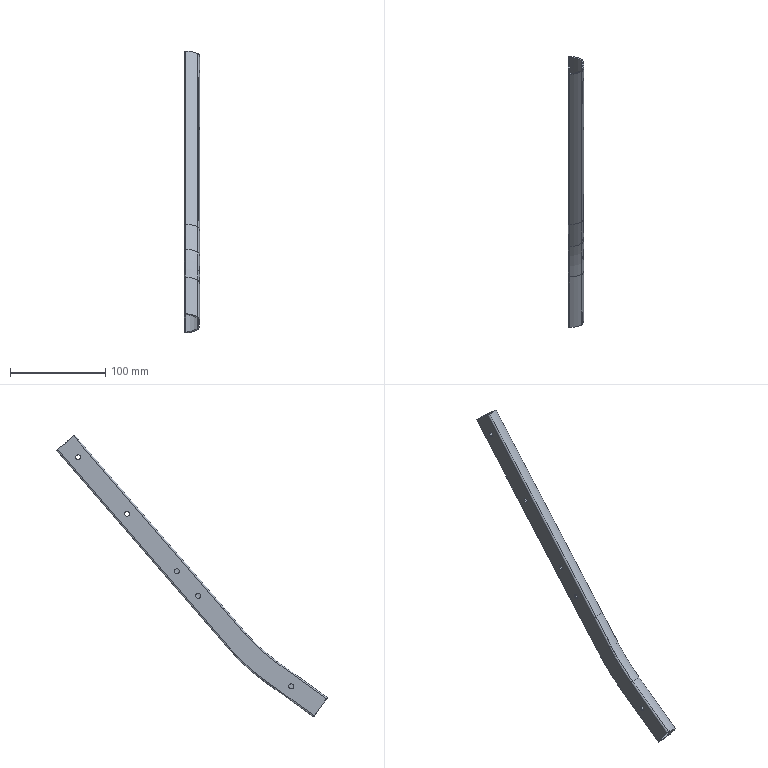Part | SolidWorks | features BaseBody 1 | 1 solid | 83 faces | box 16 x 283.583 x 295.302 mm | volume 30931 mm3 | cylinder 57 | spline 19 | plane 4 | torus 3 | commonest cylinder face diameters 5.2 x12 0.6 x8 3 x8 47.6 x6 50 x6 3.6 x5